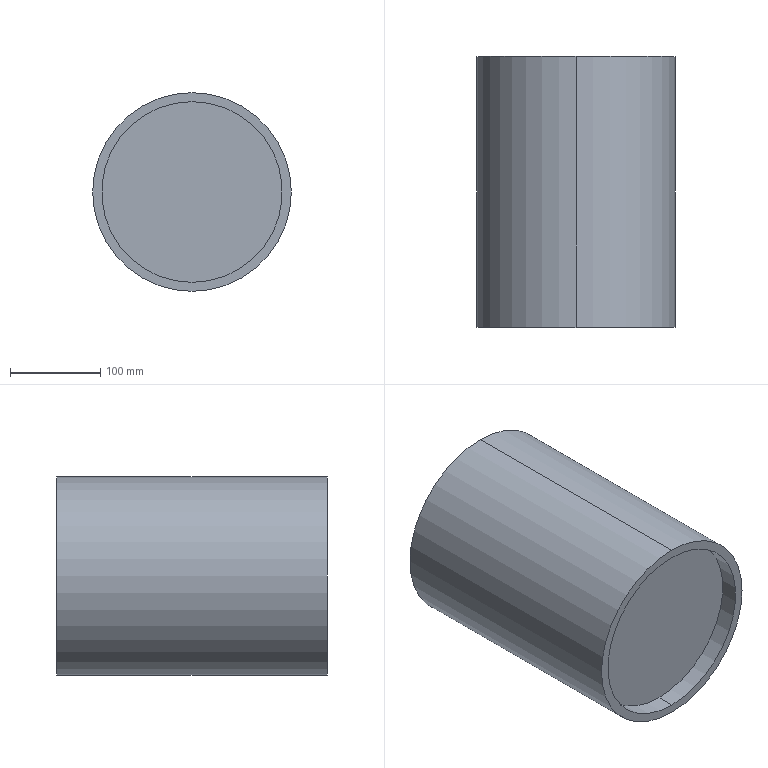Part | SolidWorks | features ICE 2, Extrusion 1 | 1 solid | 10 faces | box 220 x 300 x 220 mm | volume 2293363 mm3 | cylinder 6 | plane 4 | commonest cylinder face diameters 200 x4 220 x2
STEP:
#1=CARTESIAN_POINT('',(0.,30.,-100.));
#2=VERTEX_POINT('',#1);
#3=CARTESIAN_POINT('',(0.,30.,100.));
#4=VERTEX_POINT('',#3);
#5=CARTESIAN_POINT('',(0.,30.,0.));
#6=DIRECTION('',(0.,1.,0.));
#7=DIRECTION('',(0.,0.,1.));
#8=AXIS2_PLACEMENT_3D('',#5,#6,#7);
#9=CIRCLE('',#8,100.);
#10=EDGE_CURVE('',#2,#4,#9,.T.);
#11=ORIENTED_EDGE('',*,*,#10,.F.);
#12=CARTESIAN_POINT('',(0.,300.,-100.));
#13=VERTEX_POINT('',#12);
#14=CARTESIAN_POINT('',(0.,30.,-100.));
#15=DIRECTION('',(0.,1.,0.));
#16=VECTOR('',#15,1000.);
#17=LINE('',#14,#16);
#18=EDGE_CURVE('',#2,#13,#17,.T.);
#19=ORIENTED_EDGE('',*,*,#18,.T.);
#20=CARTESIAN_POINT('',(0.,300.,100.));
#21=VERTEX_POINT('',#20);
#22=CARTESIAN_POINT('',(0.,300.,0.));
#23=DIRECTION('',(0.,1.,0.));
#24=DIRECTION('',(0.,0.,1.));
#25=AXIS2_PLACEMENT_3D('',#22,#23,#24);
#26=CIRCLE('',#25,100.);
#27=EDGE_CURVE('',#13,#21,#26,.T.);
#28=ORIENTED_EDGE('',*,*,#27,.T.);
#29=CARTESIAN_POINT('',(0.,30.,100.));
#30=DIRECTION('',(0.,1.,0.));
#31=VECTOR('',#30,1000.);
#32=LINE('',#29,#31);
#33=EDGE_CURVE('',#4,#21,#32,.T.);
#34=ORIENTED_EDGE('',*,*,#33,.F.);
#35=EDGE_LOOP('',(#11,#19,#28,#34));
#36=FACE_OUTER_BOUND('',#35,.T.);
#37=CARTESIAN_POINT('',(0.,30.,0.));
#38=DIRECTION('',(0.,1.,0.));
#39=DIRECTION('',(0.,0.,1.));
#40=AXIS2_PLACEMENT_3D('',#37,#38,#39);
#41=CYLINDRICAL_SURFACE('',#40,100.);
#42=ADVANCED_FACE('',(#36),#41,.F.);
#43=CARTESIAN_POINT('',(0.,20.,100.));
#44=VERTEX_POINT('',#43);
#45=CARTESIAN_POINT('',(0.,20.,-100.));
#46=VERTEX_POINT('',#45);
#47=CARTESIAN_POINT('',(0.,20.,0.));
#48=DIRECTION('',(0.,-1.,0.));
#49=DIRECTION('',(0.,0.,-1.));
#50=AXIS2_PLACEMENT_3D('',#47,#48,#49);
#51=CIRCLE('',#50,100.);
#52=EDGE_CURVE('',#44,#46,#51,.T.);
#53=ORIENTED_EDGE('',*,*,#52,.F.);
#54=CARTESIAN_POINT('',(0.,0.,100.));
#55=VERTEX_POINT('',#54);
#56=CARTESIAN_POINT('',(0.,20.,100.));
#57=DIRECTION('',(0.,-1.,0.));
#58=VECTOR('',#57,1000.);
#59=LINE('',#56,#58);
#60=EDGE_CURVE('',#44,#55,#59,.T.);
#61=ORIENTED_EDGE('',*,*,#60,.T.);
#62=CARTESIAN_POINT('',(0.,0.,-100.));
#63=VERTEX_POINT('',#62);
#64=CARTESIAN_POINT('',(0.,0.,0.));
#65=DIRECTION('',(0.,-1.,0.));
#66=DIRECTION('',(0.,0.,-1.));
#67=AXIS2_PLACEMENT_3D('',#64,#65,#66);
#68=CIRCLE('',#67,100.);
#69=EDGE_CURVE('',#55,#63,#68,.T.);
#70=ORIENTED_EDGE('',*,*,#69,.T.);
#71=CARTESIAN_POINT('',(0.,20.,-100.));
#72=DIRECTION('',(0.,-1.,0.));
#73=VECTOR('',#72,1000.);
#74=LINE('',#71,#73);
#75=EDGE_CURVE('',#46,#63,#74,.T.);
#76=ORIENTED_EDGE('',*,*,#75,.F.);
#77=EDGE_LOOP('',(#53,#61,#70,#76));
#78=FACE_OUTER_BOUND('',#77,.T.);
#79=CARTESIAN_POINT('',(0.,20.,0.));
#80=DIRECTION('',(0.,-1.,0.));
#81=DIRECTION('',(0.,0.,-1.));
#82=AXIS2_PLACEMENT_3D('',#79,#80,#81);
#83=CYLINDRICAL_SURFACE('',#82,100.);
#84=ADVANCED_FACE('',(#78),#83,.F.);
#85=CARTESIAN_POINT('',(0.,300.,110.));
#86=VERTEX_POINT('',#85);
#87=CARTESIAN_POINT('',(0.,300.,-110.));
#88=VERTEX_POINT('',#87);
#89=CARTESIAN_POINT('',(0.,300.,0.));
#90=DIRECTION('',(0.,1.,0.));
#91=DIRECTION('',(0.,0.,1.));
#92=AXIS2_PLACEMENT_3D('',#89,#90,#91);
#93=CIRCLE('',#92,110.);
#94=EDGE_CURVE('',#86,#88,#93,.T.);
#95=ORIENTED_EDGE('',*,*,#94,.F.);
#96=CARTESIAN_POINT('',(0.,0.,110.));
#97=VERTEX_POINT('',#96);
#98=CARTESIAN_POINT('',(0.,300.,110.));
#99=DIRECTION('',(0.,-1.,0.));
#100=VECTOR('',#99,1000.);
#101=LINE('',#98,#100);
#102=EDGE_CURVE('',#86,#97,#101,.T.);
#103=ORIENTED_EDGE('',*,*,#102,.T.);
#104=CARTESIAN_POINT('',(0.,0.,-110.));
#105=VERTEX_POINT('',#104);
#106=CARTESIAN_POINT('',(0.,0.,0.));
#107=DIRECTION('',(0.,1.,0.));
#108=DIRECTION('',(0.,0.,1.));
#109=AXIS2_PLACEMENT_3D('',#106,#107,#108);
#110=CIRCLE('',#109,110.);
#111=EDGE_CURVE('',#97,#105,#110,.T.);
#112=ORIENTED_EDGE('',*,*,#111,.T.);
#113=CARTESIAN_POINT('',(0.,300.,-110.));
#114=DIRECTION('',(0.,-1.,0.));
#115=VECTOR('',#114,1000.);
#116=LINE('',#113,#115);
#117=EDGE_CURVE('',#88,#105,#116,.T.);
#118=ORIENTED_EDGE('',*,*,#117,.F.);
#119=EDGE_LOOP('',(#95,#103,#112,#118));
#120=FACE_OUTER_BOUND('',#119,.T.);
#121=CARTESIAN_POINT('',(0.,300.,0.));
#122=DIRECTION('',(0.,-1.,0.));
#123=DIRECTION('',(0.,0.,-1.));
#124=AXIS2_PLACEMENT_3D('',#121,#122,#123);
#125=CYLINDRICAL_SURFACE('',#124,110.);
#126=ADVANCED_FACE('',(#120),#125,.T.);
#127=ORIENTED_EDGE('',*,*,#102,.F.);
#128=CARTESIAN_POINT('',(0.,300.,0.));
#129=DIRECTION('',(0.,1.,0.));
#130=DIRECTION('',(0.,0.,1.));
#131=AXIS2_PLACEMENT_3D('',#128,#129,#130);
#132=CIRCLE('',#131,110.);
#133=EDGE_CURVE('',#88,#86,#132,.T.);
#134=ORIENTED_EDGE('',*,*,#133,.F.);
#135=ORIENTED_EDGE('',*,*,#117,.T.);
#136=CARTESIAN_POINT('',(0.,0.,0.));
#137=DIRECTION('',(0.,1.,0.));
#138=DIRECTION('',(0.,0.,1.));
#139=AXIS2_PLACEMENT_3D('',#136,#137,#138);
#140=CIRCLE('',#139,110.);
#141=EDGE_CURVE('',#105,#97,#140,.T.);
#142=ORIENTED_EDGE('',*,*,#141,.T.);
#143=EDGE_LOOP('',(#127,#134,#135,#142));
#144=FACE_OUTER_BOUND('',#143,.T.);
#145=CARTESIAN_POINT('',(0.,300.,0.));
#146=DIRECTION('',(0.,-1.,0.));
#147=DIRECTION('',(0.,0.,-1.));
#148=AXIS2_PLACEMENT_3D('',#145,#146,#147);
#149=CYLINDRICAL_SURFACE('',#148,110.);
#150=ADVANCED_FACE('',(#144),#149,.T.);
#151=CARTESIAN_POINT('',(0.,300.,0.));
#152=DIRECTION('',(0.,1.,0.));
#153=DIRECTION('',(0.,0.,1.));
#154=AXIS2_PLACEMENT_3D('',#151,#152,#153);
#155=CIRCLE('',#154,100.);
#156=EDGE_CURVE('',#21,#13,#155,.T.);
#157=ORIENTED_EDGE('',*,*,#156,.F.);
#158=ORIENTED_EDGE('',*,*,#27,.F.);
#159=EDGE_LOOP('',(#157,#158));
#160=FACE_BOUND('',#159,.T.);
#161=ORIENTED_EDGE('',*,*,#133,.T.);
#162=ORIENTED_EDGE('',*,*,#94,.T.);
#163=EDGE_LOOP('',(#161,#162));
#164=FACE_OUTER_BOUND('',#163,.T.);
#165=CARTESIAN_POINT('',(0.,300.,0.));
#166=DIRECTION('',(0.,1.,0.));
#167=DIRECTION('',(0.,0.,1.));
#168=AXIS2_PLACEMENT_3D('',#165,#166,#167);
#169=PLANE('',#168);
#170=ADVANCED_FACE('',(#160,#164),#169,.T.);
#171=CARTESIAN_POINT('',(0.,0.,0.));
#172=DIRECTION('',(0.,-1.,0.));
#173=DIRECTION('',(0.,0.,-1.));
#174=AXIS2_PLACEMENT_3D('',#171,#172,#173);
#175=CIRCLE('',#174,100.);
#176=EDGE_CURVE('',#63,#55,#175,.T.);
#177=ORIENTED_EDGE('',*,*,#176,.F.);
#178=ORIENTED_EDGE('',*,*,#69,.F.);
#179=EDGE_LOOP('',(#177,#178));
#180=FACE_BOUND('',#179,.T.);
#181=ORIENTED_EDGE('',*,*,#141,.F.);
#182=ORIENTED_EDGE('',*,*,#111,.F.);
#183=EDGE_LOOP('',(#181,#182));
#184=FACE_OUTER_BOUND('',#183,.T.);
#185=CARTESIAN_POINT('',(0.,0.,0.));
#186=DIRECTION('',(0.,1.,0.));
#187=DIRECTION('',(0.,0.,1.));
#188=AXIS2_PLACEMENT_3D('',#185,#186,#187);
#189=PLANE('',#188);
#190=ADVANCED_FACE('',(#180,#184),#189,.F.);
#191=ORIENTED_EDGE('',*,*,#60,.F.);
#192=CARTESIAN_POINT('',(0.,20.,0.));
#193=DIRECTION('',(0.,-1.,0.));
#194=DIRECTION('',(0.,0.,-1.));
#195=AXIS2_PLACEMENT_3D('',#192,#193,#194);
#196=CIRCLE('',#195,100.);
#197=EDGE_CURVE('',#46,#44,#196,.T.);
#198=ORIENTED_EDGE('',*,*,#197,.F.);
#199=ORIENTED_EDGE('',*,*,#75,.T.);
#200=ORIENTED_EDGE('',*,*,#176,.T.);
#201=EDGE_LOOP('',(#191,#198,#199,#200));
#202=FACE_OUTER_BOUND('',#201,.T.);
#203=CARTESIAN_POINT('',(0.,20.,0.));
#204=DIRECTION('',(0.,-1.,0.));
#205=DIRECTION('',(0.,0.,-1.));
#206=AXIS2_PLACEMENT_3D('',#203,#204,#205);
#207=CYLINDRICAL_SURFACE('',#206,100.);
#208=ADVANCED_FACE('',(#202),#207,.F.);
#209=ORIENTED_EDGE('',*,*,#197,.T.);
#210=ORIENTED_EDGE('',*,*,#52,.T.);
#211=EDGE_LOOP('',(#209,#210));
#212=FACE_OUTER_BOUND('',#211,.T.);
#213=CARTESIAN_POINT('',(0.,20.,0.));
#214=DIRECTION('',(0.,-1.,0.));
#215=DIRECTION('',(0.,0.,-1.));
#216=AXIS2_PLACEMENT_3D('',#213,#214,#215);
#217=PLANE('',#216);
#218=ADVANCED_FACE('',(#212),#217,.T.);
#219=ORIENTED_EDGE('',*,*,#18,.F.);
#220=CARTESIAN_POINT('',(0.,30.,0.));
#221=DIRECTION('',(0.,1.,0.));
#222=DIRECTION('',(0.,0.,1.));
#223=AXIS2_PLACEMENT_3D('',#220,#221,#222);
#224=CIRCLE('',#223,100.);
#225=EDGE_CURVE('',#4,#2,#224,.T.);
#226=ORIENTED_EDGE('',*,*,#225,.F.);
#227=ORIENTED_EDGE('',*,*,#33,.T.);
#228=ORIENTED_EDGE('',*,*,#156,.T.);
#229=EDGE_LOOP('',(#219,#226,#227,#228));
#230=FACE_OUTER_BOUND('',#229,.T.);
#231=CARTESIAN_POINT('',(0.,30.,0.));
#232=DIRECTION('',(0.,1.,0.));
#233=DIRECTION('',(0.,0.,1.));
#234=AXIS2_PLACEMENT_3D('',#231,#232,#233);
#235=CYLINDRICAL_SURFACE('',#234,100.);
#236=ADVANCED_FACE('',(#230),#235,.F.);
#237=ORIENTED_EDGE('',*,*,#225,.T.);
#238=ORIENTED_EDGE('',*,*,#10,.T.);
#239=EDGE_LOOP('',(#237,#238));
#240=FACE_OUTER_BOUND('',#239,.T.);
#241=CARTESIAN_POINT('',(0.,30.,0.));
#242=DIRECTION('',(0.,1.,0.));
#243=DIRECTION('',(0.,0.,1.));
#244=AXIS2_PLACEMENT_3D('',#241,#242,#243);
#245=PLANE('',#244);
#246=ADVANCED_FACE('',(#240),#245,.T.);
#247=CLOSED_SHELL('',(#42,#84,#126,#150,#170,#190,#208,#218,#236,#246));
#248=MANIFOLD_SOLID_BREP('',#247);
#249=CARTESIAN_POINT('',(0.,0.,0.));
#250=DIRECTION('',(0.,0.,1.));
#251=DIRECTION('',(1.,0.,0.));
#252=AXIS2_PLACEMENT_3D('',#249,#250,#251);
#253=(LENGTH_UNIT()NAMED_UNIT(*)SI_UNIT(.MILLI.,.METRE.));
#254=UNCERTAINTY_MEASURE_WITH_UNIT(LENGTH_MEASURE(0.00001),#253,'','');
#255=(NAMED_UNIT(*)PLANE_ANGLE_UNIT()SI_UNIT($,.RADIAN.));
#256=(NAMED_UNIT(*)SI_UNIT($,.STERADIAN.)SOLID_ANGLE_UNIT());
#257=(GEOMETRIC_REPRESENTATION_CONTEXT(3)GLOBAL_UNCERTAINTY_ASSIGNED_CONTEXT((#254))GLOBAL_UNIT_ASSIGNED_CONTEXT((#253,#255,#256))REPRESENTATION_CONTEXT('',''));
#258=ADVANCED_BREP_SHAPE_REPRESENTATION('',(#248,#252),#257);